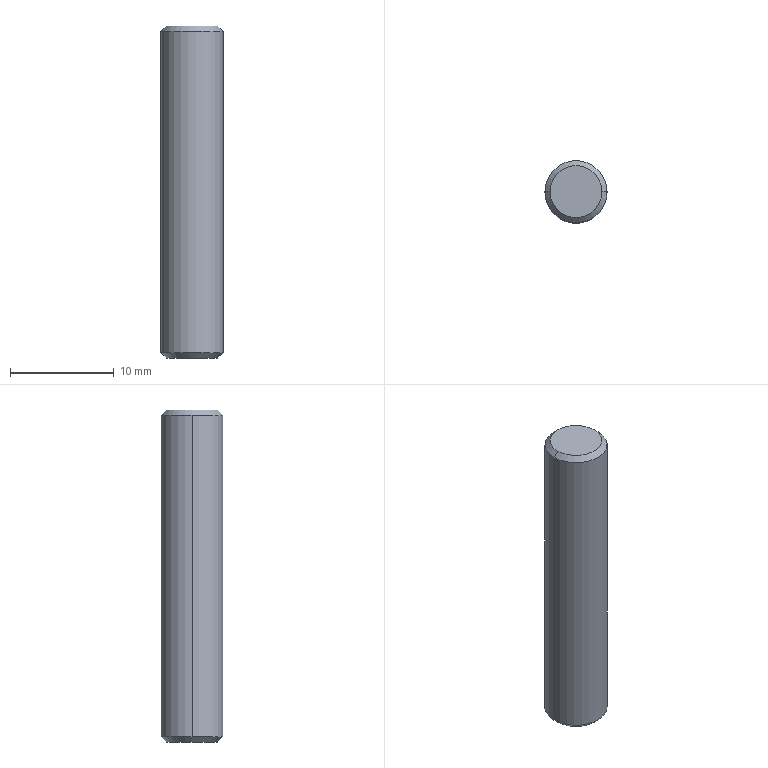Part | SolidWorks | features Chamfer 1, Extrusion 1 | 1 solid | 8 faces | box 6 x 6 x 32 mm | volume 900.328 mm3 | cone 4 | cylinder 2 | plane 2 | commonest cylinder face diameters 6 x2
STEP:
#1=CARTESIAN_POINT('',(-2.5,0.,0.));
#2=VERTEX_POINT('',#1);
#3=CARTESIAN_POINT('',(2.5,0.,0.));
#4=VERTEX_POINT('',#3);
#5=CARTESIAN_POINT('',(0.,0.,0.));
#6=DIRECTION('',(0.,0.,-1.));
#7=DIRECTION('',(1.,0.,0.));
#8=AXIS2_PLACEMENT_3D('',#5,#6,#7);
#9=CIRCLE('',#8,2.5);
#10=EDGE_CURVE('',#2,#4,#9,.T.);
#11=ORIENTED_EDGE('',*,*,#10,.F.);
#12=CARTESIAN_POINT('',(-3.,0.,0.5));
#13=VERTEX_POINT('',#12);
#14=CARTESIAN_POINT('',(-3.,0.,0.5));
#15=DIRECTION('',(-0.7071,0.,0.7071));
#16=VECTOR('',#15,1000.);
#17=LINE('',#14,#16);
#18=EDGE_CURVE('',#2,#13,#17,.T.);
#19=ORIENTED_EDGE('',*,*,#18,.T.);
#20=CARTESIAN_POINT('',(3.,0.,0.5));
#21=VERTEX_POINT('',#20);
#22=CARTESIAN_POINT('',(0.,0.,0.5));
#23=DIRECTION('',(0.,0.,1.));
#24=DIRECTION('',(1.,0.,0.));
#25=AXIS2_PLACEMENT_3D('',#22,#23,#24);
#26=CIRCLE('',#25,3.);
#27=EDGE_CURVE('',#21,#13,#26,.T.);
#28=ORIENTED_EDGE('',*,*,#27,.F.);
#29=CARTESIAN_POINT('',(3.,0.,0.5));
#30=DIRECTION('',(0.7071,0.,0.7071));
#31=VECTOR('',#30,1000.);
#32=LINE('',#29,#31);
#33=EDGE_CURVE('',#4,#21,#32,.T.);
#34=ORIENTED_EDGE('',*,*,#33,.F.);
#35=EDGE_LOOP('',(#11,#19,#28,#34));
#36=FACE_OUTER_BOUND('',#35,.T.);
#37=CARTESIAN_POINT('',(0.,0.,0.5));
#38=DIRECTION('',(0.,0.,1.));
#39=DIRECTION('',(1.,0.,0.));
#40=AXIS2_PLACEMENT_3D('',#37,#38,#39);
#41=CONICAL_SURFACE('',#40,3.,0.7854);
#42=ADVANCED_FACE('',(#36),#41,.T.);
#43=CARTESIAN_POINT('',(2.5,0.,32.));
#44=VERTEX_POINT('',#43);
#45=CARTESIAN_POINT('',(-2.5,0.,32.));
#46=VERTEX_POINT('',#45);
#47=CARTESIAN_POINT('',(0.,0.,32.));
#48=DIRECTION('',(0.,0.,1.));
#49=DIRECTION('',(1.,0.,0.));
#50=AXIS2_PLACEMENT_3D('',#47,#48,#49);
#51=CIRCLE('',#50,2.5);
#52=EDGE_CURVE('',#44,#46,#51,.T.);
#53=ORIENTED_EDGE('',*,*,#52,.F.);
#54=CARTESIAN_POINT('',(3.,0.,31.5));
#55=VERTEX_POINT('',#54);
#56=CARTESIAN_POINT('',(2.5,0.,32.));
#57=DIRECTION('',(0.7071,0.,-0.7071));
#58=VECTOR('',#57,1000.);
#59=LINE('',#56,#58);
#60=EDGE_CURVE('',#44,#55,#59,.T.);
#61=ORIENTED_EDGE('',*,*,#60,.T.);
#62=CARTESIAN_POINT('',(-3.,0.,31.5));
#63=VERTEX_POINT('',#62);
#64=CARTESIAN_POINT('',(0.,0.,31.5));
#65=DIRECTION('',(0.,0.,-1.));
#66=DIRECTION('',(1.,0.,0.));
#67=AXIS2_PLACEMENT_3D('',#64,#65,#66);
#68=CIRCLE('',#67,3.);
#69=EDGE_CURVE('',#63,#55,#68,.T.);
#70=ORIENTED_EDGE('',*,*,#69,.F.);
#71=CARTESIAN_POINT('',(-2.5,0.,32.));
#72=DIRECTION('',(-0.7071,0.,-0.7071));
#73=VECTOR('',#72,1000.);
#74=LINE('',#71,#73);
#75=EDGE_CURVE('',#46,#63,#74,.T.);
#76=ORIENTED_EDGE('',*,*,#75,.F.);
#77=EDGE_LOOP('',(#53,#61,#70,#76));
#78=FACE_OUTER_BOUND('',#77,.T.);
#79=CARTESIAN_POINT('',(0.,0.,32.));
#80=DIRECTION('',(0.,0.,-1.));
#81=DIRECTION('',(-1.,0.,0.));
#82=AXIS2_PLACEMENT_3D('',#79,#80,#81);
#83=CONICAL_SURFACE('',#82,2.5,0.7854);
#84=ADVANCED_FACE('',(#78),#83,.T.);
#85=ORIENTED_EDGE('',*,*,#69,.T.);
#86=CARTESIAN_POINT('',(3.,0.,32.));
#87=DIRECTION('',(0.,0.,-1.));
#88=VECTOR('',#87,1000.);
#89=LINE('',#86,#88);
#90=EDGE_CURVE('',#55,#21,#89,.T.);
#91=ORIENTED_EDGE('',*,*,#90,.T.);
#92=ORIENTED_EDGE('',*,*,#27,.T.);
#93=CARTESIAN_POINT('',(-3.,0.,32.));
#94=DIRECTION('',(0.,0.,-1.));
#95=VECTOR('',#94,1000.);
#96=LINE('',#93,#95);
#97=EDGE_CURVE('',#63,#13,#96,.T.);
#98=ORIENTED_EDGE('',*,*,#97,.F.);
#99=EDGE_LOOP('',(#85,#91,#92,#98));
#100=FACE_OUTER_BOUND('',#99,.T.);
#101=CARTESIAN_POINT('',(0.,0.,32.));
#102=DIRECTION('',(0.,0.,-1.));
#103=DIRECTION('',(-1.,0.,0.));
#104=AXIS2_PLACEMENT_3D('',#101,#102,#103);
#105=CYLINDRICAL_SURFACE('',#104,3.);
#106=ADVANCED_FACE('',(#100),#105,.T.);
#107=ORIENTED_EDGE('',*,*,#90,.F.);
#108=CARTESIAN_POINT('',(0.,0.,31.5));
#109=DIRECTION('',(0.,0.,-1.));
#110=DIRECTION('',(1.,0.,0.));
#111=AXIS2_PLACEMENT_3D('',#108,#109,#110);
#112=CIRCLE('',#111,3.);
#113=EDGE_CURVE('',#55,#63,#112,.T.);
#114=ORIENTED_EDGE('',*,*,#113,.T.);
#115=ORIENTED_EDGE('',*,*,#97,.T.);
#116=CARTESIAN_POINT('',(0.,0.,0.5));
#117=DIRECTION('',(0.,0.,1.));
#118=DIRECTION('',(1.,0.,0.));
#119=AXIS2_PLACEMENT_3D('',#116,#117,#118);
#120=CIRCLE('',#119,3.);
#121=EDGE_CURVE('',#13,#21,#120,.T.);
#122=ORIENTED_EDGE('',*,*,#121,.T.);
#123=EDGE_LOOP('',(#107,#114,#115,#122));
#124=FACE_OUTER_BOUND('',#123,.T.);
#125=CARTESIAN_POINT('',(0.,0.,32.));
#126=DIRECTION('',(0.,0.,-1.));
#127=DIRECTION('',(-1.,0.,0.));
#128=AXIS2_PLACEMENT_3D('',#125,#126,#127);
#129=CYLINDRICAL_SURFACE('',#128,3.);
#130=ADVANCED_FACE('',(#124),#129,.T.);
#131=CARTESIAN_POINT('',(0.,0.,32.));
#132=DIRECTION('',(0.,0.,1.));
#133=DIRECTION('',(1.,0.,0.));
#134=AXIS2_PLACEMENT_3D('',#131,#132,#133);
#135=CIRCLE('',#134,2.5);
#136=EDGE_CURVE('',#46,#44,#135,.T.);
#137=ORIENTED_EDGE('',*,*,#136,.T.);
#138=ORIENTED_EDGE('',*,*,#52,.T.);
#139=EDGE_LOOP('',(#137,#138));
#140=FACE_OUTER_BOUND('',#139,.T.);
#141=CARTESIAN_POINT('',(0.,0.,32.));
#142=DIRECTION('',(0.,0.,1.));
#143=DIRECTION('',(1.,0.,0.));
#144=AXIS2_PLACEMENT_3D('',#141,#142,#143);
#145=PLANE('',#144);
#146=ADVANCED_FACE('',(#140),#145,.T.);
#147=CARTESIAN_POINT('',(0.,0.,0.));
#148=DIRECTION('',(0.,0.,-1.));
#149=DIRECTION('',(1.,0.,0.));
#150=AXIS2_PLACEMENT_3D('',#147,#148,#149);
#151=CIRCLE('',#150,2.5);
#152=EDGE_CURVE('',#4,#2,#151,.T.);
#153=ORIENTED_EDGE('',*,*,#152,.T.);
#154=ORIENTED_EDGE('',*,*,#10,.T.);
#155=EDGE_LOOP('',(#153,#154));
#156=FACE_OUTER_BOUND('',#155,.T.);
#157=CARTESIAN_POINT('',(0.,0.,0.));
#158=DIRECTION('',(0.,0.,1.));
#159=DIRECTION('',(1.,0.,0.));
#160=AXIS2_PLACEMENT_3D('',#157,#158,#159);
#161=PLANE('',#160);
#162=ADVANCED_FACE('',(#156),#161,.F.);
#163=ORIENTED_EDGE('',*,*,#60,.F.);
#164=ORIENTED_EDGE('',*,*,#136,.F.);
#165=ORIENTED_EDGE('',*,*,#75,.T.);
#166=ORIENTED_EDGE('',*,*,#113,.F.);
#167=EDGE_LOOP('',(#163,#164,#165,#166));
#168=FACE_OUTER_BOUND('',#167,.T.);
#169=CARTESIAN_POINT('',(0.,0.,32.));
#170=DIRECTION('',(0.,0.,-1.));
#171=DIRECTION('',(-1.,0.,0.));
#172=AXIS2_PLACEMENT_3D('',#169,#170,#171);
#173=CONICAL_SURFACE('',#172,2.5,0.7854);
#174=ADVANCED_FACE('',(#168),#173,.T.);
#175=ORIENTED_EDGE('',*,*,#18,.F.);
#176=ORIENTED_EDGE('',*,*,#152,.F.);
#177=ORIENTED_EDGE('',*,*,#33,.T.);
#178=ORIENTED_EDGE('',*,*,#121,.F.);
#179=EDGE_LOOP('',(#175,#176,#177,#178));
#180=FACE_OUTER_BOUND('',#179,.T.);
#181=CARTESIAN_POINT('',(0.,0.,0.5));
#182=DIRECTION('',(0.,0.,1.));
#183=DIRECTION('',(1.,0.,0.));
#184=AXIS2_PLACEMENT_3D('',#181,#182,#183);
#185=CONICAL_SURFACE('',#184,3.,0.7854);
#186=ADVANCED_FACE('',(#180),#185,.T.);
#187=CLOSED_SHELL('',(#42,#84,#106,#130,#146,#162,#174,#186));
#188=MANIFOLD_SOLID_BREP('',#187);
#189=CARTESIAN_POINT('',(0.,0.,0.));
#190=DIRECTION('',(0.,0.,1.));
#191=DIRECTION('',(1.,0.,0.));
#192=AXIS2_PLACEMENT_3D('',#189,#190,#191);
#193=(LENGTH_UNIT()NAMED_UNIT(*)SI_UNIT(.MILLI.,.METRE.));
#194=UNCERTAINTY_MEASURE_WITH_UNIT(LENGTH_MEASURE(0.00001),#193,'','');
#195=(NAMED_UNIT(*)PLANE_ANGLE_UNIT()SI_UNIT($,.RADIAN.));
#196=(NAMED_UNIT(*)SI_UNIT($,.STERADIAN.)SOLID_ANGLE_UNIT());
#197=(GEOMETRIC_REPRESENTATION_CONTEXT(3)GLOBAL_UNCERTAINTY_ASSIGNED_CONTEXT((#194))GLOBAL_UNIT_ASSIGNED_CONTEXT((#193,#195,#196))REPRESENTATION_CONTEXT('',''));
#198=ADVANCED_BREP_SHAPE_REPRESENTATION('',(#188,#192),#197);